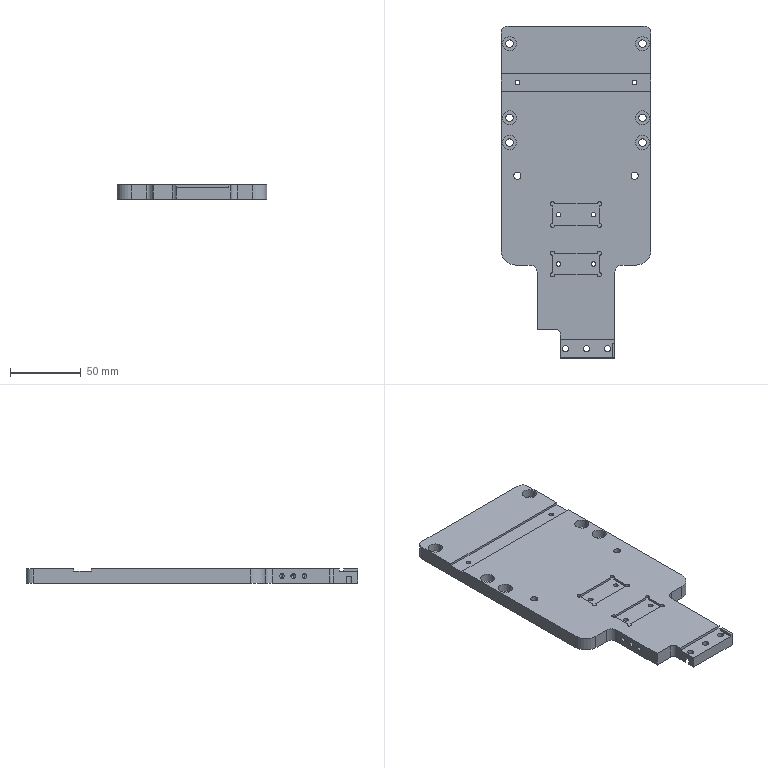Part | SolidWorks | features ICE 18, HoleWzd 12, Fillet 5, MoveFace 3, LPattern 2, MirrorPattern 2, Extrusion 1 | 1 solid | 134 faces | box 106 x 235 x 10 mm | volume 201663 mm3 | cylinder 82 | plane 40 | cone 12 | commonest cylinder face diameters 3.3 x24 10 x16 3 x12 5.4 x12 4.4 x6 8 x5